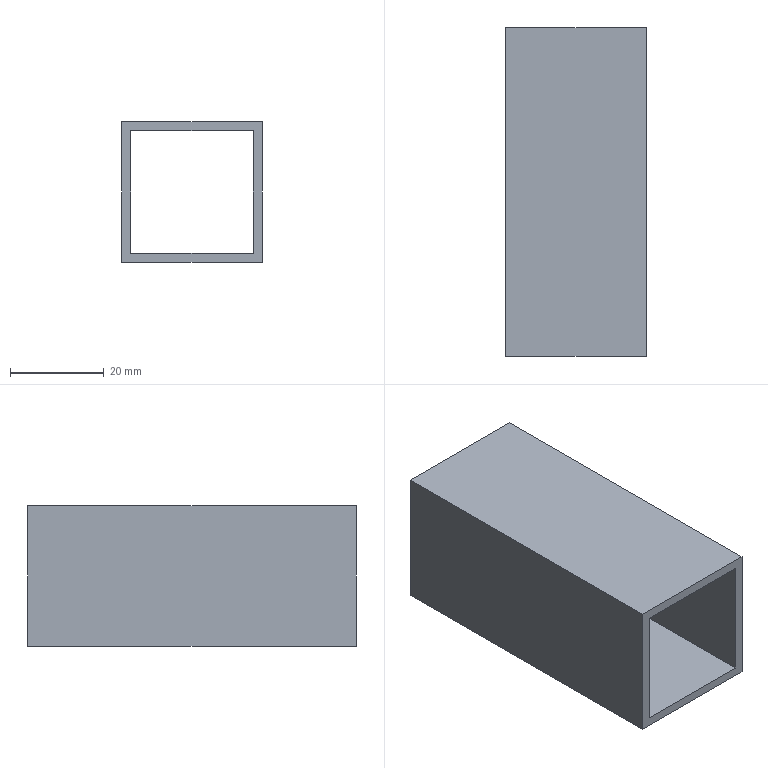Part | NX | features solid 2 | 1 solid | 10 faces | box 30 x 70 x 30 mm | volume 15680 mm3 | plane 10
STEP:
#1=CARTESIAN_POINT('',(245.839,786.479,-180.));
#2=VERTEX_POINT('',#1);
#3=CARTESIAN_POINT('',(245.839,786.479,-150.));
#4=VERTEX_POINT('',#3);
#5=CARTESIAN_POINT('',(245.839,786.479,-180.));
#6=DIRECTION('',(0.,0.,1.));
#7=VECTOR('',#6,1000.);
#8=LINE('',#5,#7);
#9=EDGE_CURVE('',#2,#4,#8,.T.);
#10=ORIENTED_EDGE('',*,*,#9,.F.);
#11=CARTESIAN_POINT('',(245.839,716.479,-180.));
#12=VERTEX_POINT('',#11);
#13=CARTESIAN_POINT('',(245.839,776.479,-180.));
#14=DIRECTION('',(0.,1.,0.));
#15=VECTOR('',#14,1000.);
#16=LINE('',#13,#15);
#17=EDGE_CURVE('',#12,#2,#16,.T.);
#18=ORIENTED_EDGE('',*,*,#17,.F.);
#19=CARTESIAN_POINT('',(245.839,716.479,-150.));
#20=VERTEX_POINT('',#19);
#21=CARTESIAN_POINT('',(245.839,716.479,-180.));
#22=DIRECTION('',(0.,0.,-1.));
#23=VECTOR('',#22,1000.);
#24=LINE('',#21,#23);
#25=EDGE_CURVE('',#12,#20,#24,.F.);
#26=ORIENTED_EDGE('',*,*,#25,.T.);
#27=CARTESIAN_POINT('',(245.839,776.479,-150.));
#28=DIRECTION('',(0.,1.,0.));
#29=VECTOR('',#28,1000.);
#30=LINE('',#27,#29);
#31=EDGE_CURVE('',#20,#4,#30,.T.);
#32=ORIENTED_EDGE('',*,*,#31,.T.);
#33=EDGE_LOOP('',(#10,#18,#26,#32));
#34=FACE_BOUND('',#33,.T.);
#35=CARTESIAN_POINT('',(245.839,776.479,-180.));
#36=DIRECTION('',(1.,0.,0.));
#37=DIRECTION('',(0.,1.,0.));
#38=AXIS2_PLACEMENT_3D('',#35,#36,#37);
#39=PLANE('',#38);
#40=ADVANCED_FACE('',(#34),#39,.F.);
#41=CARTESIAN_POINT('',(275.839,786.479,-150.));
#42=VERTEX_POINT('',#41);
#43=CARTESIAN_POINT('',(275.839,786.479,-180.));
#44=VERTEX_POINT('',#43);
#45=CARTESIAN_POINT('',(275.839,786.479,-180.));
#46=DIRECTION('',(0.,0.,1.));
#47=VECTOR('',#46,1000.);
#48=LINE('',#45,#47);
#49=EDGE_CURVE('',#42,#44,#48,.F.);
#50=ORIENTED_EDGE('',*,*,#49,.F.);
#51=CARTESIAN_POINT('',(275.839,716.479,-150.));
#52=VERTEX_POINT('',#51);
#53=CARTESIAN_POINT('',(275.839,776.479,-150.));
#54=DIRECTION('',(0.,-1.,0.));
#55=VECTOR('',#54,1000.);
#56=LINE('',#53,#55);
#57=EDGE_CURVE('',#52,#42,#56,.F.);
#58=ORIENTED_EDGE('',*,*,#57,.F.);
#59=CARTESIAN_POINT('',(275.839,716.479,-180.));
#60=VERTEX_POINT('',#59);
#61=CARTESIAN_POINT('',(275.839,716.479,-180.));
#62=DIRECTION('',(0.,0.,-1.));
#63=VECTOR('',#62,1000.);
#64=LINE('',#61,#63);
#65=EDGE_CURVE('',#52,#60,#64,.T.);
#66=ORIENTED_EDGE('',*,*,#65,.T.);
#67=CARTESIAN_POINT('',(275.839,776.479,-180.));
#68=DIRECTION('',(0.,1.,0.));
#69=VECTOR('',#68,1000.);
#70=LINE('',#67,#69);
#71=EDGE_CURVE('',#60,#44,#70,.T.);
#72=ORIENTED_EDGE('',*,*,#71,.T.);
#73=EDGE_LOOP('',(#50,#58,#66,#72));
#74=FACE_BOUND('',#73,.T.);
#75=CARTESIAN_POINT('',(275.839,776.479,-180.));
#76=DIRECTION('',(1.,0.,0.));
#77=DIRECTION('',(0.,1.,0.));
#78=AXIS2_PLACEMENT_3D('',#75,#76,#77);
#79=PLANE('',#78);
#80=ADVANCED_FACE('',(#74),#79,.T.);
#81=CARTESIAN_POINT('',(275.839,786.479,-180.));
#82=DIRECTION('',(-1.,0.,0.));
#83=VECTOR('',#82,1000.);
#84=LINE('',#81,#83);
#85=EDGE_CURVE('',#44,#2,#84,.T.);
#86=ORIENTED_EDGE('',*,*,#85,.F.);
#87=ORIENTED_EDGE('',*,*,#71,.F.);
#88=CARTESIAN_POINT('',(275.839,716.479,-180.));
#89=DIRECTION('',(1.,0.,0.));
#90=VECTOR('',#89,1000.);
#91=LINE('',#88,#90);
#92=EDGE_CURVE('',#60,#12,#91,.F.);
#93=ORIENTED_EDGE('',*,*,#92,.T.);
#94=ORIENTED_EDGE('',*,*,#17,.T.);
#95=EDGE_LOOP('',(#86,#87,#93,#94));
#96=FACE_BOUND('',#95,.T.);
#97=CARTESIAN_POINT('',(275.839,776.479,-180.));
#98=DIRECTION('',(0.,0.,1.));
#99=DIRECTION('',(0.,-1.,0.));
#100=AXIS2_PLACEMENT_3D('',#97,#98,#99);
#101=PLANE('',#100);
#102=ADVANCED_FACE('',(#96),#101,.F.);
#103=ORIENTED_EDGE('',*,*,#57,.T.);
#104=CARTESIAN_POINT('',(275.839,786.479,-150.));
#105=DIRECTION('',(-1.,0.,0.));
#106=VECTOR('',#105,1000.);
#107=LINE('',#104,#106);
#108=EDGE_CURVE('',#42,#4,#107,.T.);
#109=ORIENTED_EDGE('',*,*,#108,.T.);
#110=ORIENTED_EDGE('',*,*,#31,.F.);
#111=CARTESIAN_POINT('',(275.839,716.479,-150.));
#112=DIRECTION('',(1.,0.,0.));
#113=VECTOR('',#112,1000.);
#114=LINE('',#111,#113);
#115=EDGE_CURVE('',#52,#20,#114,.F.);
#116=ORIENTED_EDGE('',*,*,#115,.F.);
#117=EDGE_LOOP('',(#103,#109,#110,#116));
#118=FACE_BOUND('',#117,.T.);
#119=CARTESIAN_POINT('',(275.839,776.479,-150.));
#120=DIRECTION('',(0.,0.,1.));
#121=DIRECTION('',(0.,-1.,0.));
#122=AXIS2_PLACEMENT_3D('',#119,#120,#121);
#123=PLANE('',#122);
#124=ADVANCED_FACE('',(#118),#123,.T.);
#125=ORIENTED_EDGE('',*,*,#115,.T.);
#126=ORIENTED_EDGE('',*,*,#25,.F.);
#127=ORIENTED_EDGE('',*,*,#92,.F.);
#128=ORIENTED_EDGE('',*,*,#65,.F.);
#129=EDGE_LOOP('',(#125,#126,#127,#128));
#130=FACE_BOUND('',#129,.T.);
#131=CARTESIAN_POINT('',(273.839,716.479,-152.));
#132=VERTEX_POINT('',#131);
#133=CARTESIAN_POINT('',(273.839,716.479,-178.));
#134=VERTEX_POINT('',#133);
#135=CARTESIAN_POINT('',(273.839,716.479,-180.));
#136=DIRECTION('',(0.,0.,-1.));
#137=VECTOR('',#136,1000.);
#138=LINE('',#135,#137);
#139=EDGE_CURVE('',#132,#134,#138,.T.);
#140=ORIENTED_EDGE('',*,*,#139,.T.);
#141=CARTESIAN_POINT('',(247.839,716.479,-178.));
#142=VERTEX_POINT('',#141);
#143=CARTESIAN_POINT('',(275.839,716.479,-178.));
#144=DIRECTION('',(1.,0.,0.));
#145=VECTOR('',#144,1000.);
#146=LINE('',#143,#145);
#147=EDGE_CURVE('',#134,#142,#146,.F.);
#148=ORIENTED_EDGE('',*,*,#147,.T.);
#149=CARTESIAN_POINT('',(247.839,716.479,-152.));
#150=VERTEX_POINT('',#149);
#151=CARTESIAN_POINT('',(247.839,716.479,-180.));
#152=DIRECTION('',(0.,0.,-1.));
#153=VECTOR('',#152,1000.);
#154=LINE('',#151,#153);
#155=EDGE_CURVE('',#142,#150,#154,.F.);
#156=ORIENTED_EDGE('',*,*,#155,.T.);
#157=CARTESIAN_POINT('',(275.839,716.479,-152.));
#158=DIRECTION('',(1.,0.,0.));
#159=VECTOR('',#158,1000.);
#160=LINE('',#157,#159);
#161=EDGE_CURVE('',#132,#150,#160,.F.);
#162=ORIENTED_EDGE('',*,*,#161,.F.);
#163=EDGE_LOOP('',(#140,#148,#156,#162));
#164=FACE_BOUND('',#163,.T.);
#165=CARTESIAN_POINT('',(275.839,716.479,-25.));
#166=DIRECTION('',(0.,-1.,0.));
#167=DIRECTION('',(1.,0.,0.));
#168=AXIS2_PLACEMENT_3D('',#165,#166,#167);
#169=PLANE('',#168);
#170=ADVANCED_FACE('',(#130,#164),#169,.T.);
#171=CARTESIAN_POINT('',(247.839,786.479,-178.));
#172=VERTEX_POINT('',#171);
#173=CARTESIAN_POINT('',(247.839,776.479,-178.));
#174=DIRECTION('',(0.,1.,0.));
#175=VECTOR('',#174,1000.);
#176=LINE('',#173,#175);
#177=EDGE_CURVE('',#142,#172,#176,.T.);
#178=ORIENTED_EDGE('',*,*,#177,.T.);
#179=CARTESIAN_POINT('',(247.839,786.479,-152.));
#180=VERTEX_POINT('',#179);
#181=CARTESIAN_POINT('',(247.839,786.479,-180.));
#182=DIRECTION('',(0.,0.,1.));
#183=VECTOR('',#182,1000.);
#184=LINE('',#181,#183);
#185=EDGE_CURVE('',#172,#180,#184,.T.);
#186=ORIENTED_EDGE('',*,*,#185,.T.);
#187=CARTESIAN_POINT('',(247.839,776.479,-152.));
#188=DIRECTION('',(0.,1.,0.));
#189=VECTOR('',#188,1000.);
#190=LINE('',#187,#189);
#191=EDGE_CURVE('',#150,#180,#190,.T.);
#192=ORIENTED_EDGE('',*,*,#191,.F.);
#193=ORIENTED_EDGE('',*,*,#155,.F.);
#194=EDGE_LOOP('',(#178,#186,#192,#193));
#195=FACE_BOUND('',#194,.T.);
#196=CARTESIAN_POINT('',(247.839,776.479,-180.));
#197=DIRECTION('',(1.,0.,0.));
#198=DIRECTION('',(0.,1.,0.));
#199=AXIS2_PLACEMENT_3D('',#196,#197,#198);
#200=PLANE('',#199);
#201=ADVANCED_FACE('',(#195),#200,.T.);
#202=CARTESIAN_POINT('',(273.839,786.479,-152.));
#203=VERTEX_POINT('',#202);
#204=CARTESIAN_POINT('',(273.839,776.479,-152.));
#205=DIRECTION('',(0.,-1.,0.));
#206=VECTOR('',#205,1000.);
#207=LINE('',#204,#206);
#208=EDGE_CURVE('',#132,#203,#207,.F.);
#209=ORIENTED_EDGE('',*,*,#208,.T.);
#210=CARTESIAN_POINT('',(273.839,786.479,-178.));
#211=VERTEX_POINT('',#210);
#212=CARTESIAN_POINT('',(273.839,786.479,-180.));
#213=DIRECTION('',(0.,0.,1.));
#214=VECTOR('',#213,1000.);
#215=LINE('',#212,#214);
#216=EDGE_CURVE('',#203,#211,#215,.F.);
#217=ORIENTED_EDGE('',*,*,#216,.T.);
#218=CARTESIAN_POINT('',(273.839,776.479,-178.));
#219=DIRECTION('',(0.,-1.,0.));
#220=VECTOR('',#219,1000.);
#221=LINE('',#218,#220);
#222=EDGE_CURVE('',#134,#211,#221,.F.);
#223=ORIENTED_EDGE('',*,*,#222,.F.);
#224=ORIENTED_EDGE('',*,*,#139,.F.);
#225=EDGE_LOOP('',(#209,#217,#223,#224));
#226=FACE_BOUND('',#225,.T.);
#227=CARTESIAN_POINT('',(273.839,776.479,-180.));
#228=DIRECTION('',(1.,0.,0.));
#229=DIRECTION('',(0.,1.,0.));
#230=AXIS2_PLACEMENT_3D('',#227,#228,#229);
#231=PLANE('',#230);
#232=ADVANCED_FACE('',(#226),#231,.F.);
#233=ORIENTED_EDGE('',*,*,#222,.T.);
#234=CARTESIAN_POINT('',(275.839,786.479,-178.));
#235=DIRECTION('',(-1.,0.,0.));
#236=VECTOR('',#235,1000.);
#237=LINE('',#234,#236);
#238=EDGE_CURVE('',#211,#172,#237,.T.);
#239=ORIENTED_EDGE('',*,*,#238,.T.);
#240=ORIENTED_EDGE('',*,*,#177,.F.);
#241=ORIENTED_EDGE('',*,*,#147,.F.);
#242=EDGE_LOOP('',(#233,#239,#240,#241));
#243=FACE_BOUND('',#242,.T.);
#244=CARTESIAN_POINT('',(275.839,776.479,-178.));
#245=DIRECTION('',(0.,0.,1.));
#246=DIRECTION('',(0.,-1.,0.));
#247=AXIS2_PLACEMENT_3D('',#244,#245,#246);
#248=PLANE('',#247);
#249=ADVANCED_FACE('',(#243),#248,.T.);
#250=CARTESIAN_POINT('',(275.839,786.479,-152.));
#251=DIRECTION('',(-1.,0.,0.));
#252=VECTOR('',#251,1000.);
#253=LINE('',#250,#252);
#254=EDGE_CURVE('',#203,#180,#253,.T.);
#255=ORIENTED_EDGE('',*,*,#254,.F.);
#256=ORIENTED_EDGE('',*,*,#208,.F.);
#257=ORIENTED_EDGE('',*,*,#161,.T.);
#258=ORIENTED_EDGE('',*,*,#191,.T.);
#259=EDGE_LOOP('',(#255,#256,#257,#258));
#260=FACE_BOUND('',#259,.T.);
#261=CARTESIAN_POINT('',(275.839,776.479,-152.));
#262=DIRECTION('',(0.,0.,1.));
#263=DIRECTION('',(0.,-1.,0.));
#264=AXIS2_PLACEMENT_3D('',#261,#262,#263);
#265=PLANE('',#264);
#266=ADVANCED_FACE('',(#260),#265,.F.);
#267=ORIENTED_EDGE('',*,*,#185,.F.);
#268=ORIENTED_EDGE('',*,*,#238,.F.);
#269=ORIENTED_EDGE('',*,*,#216,.F.);
#270=ORIENTED_EDGE('',*,*,#254,.T.);
#271=EDGE_LOOP('',(#267,#268,#269,#270));
#272=FACE_BOUND('',#271,.T.);
#273=ORIENTED_EDGE('',*,*,#85,.T.);
#274=ORIENTED_EDGE('',*,*,#9,.T.);
#275=ORIENTED_EDGE('',*,*,#108,.F.);
#276=ORIENTED_EDGE('',*,*,#49,.T.);
#277=EDGE_LOOP('',(#273,#274,#275,#276));
#278=FACE_BOUND('',#277,.T.);
#279=CARTESIAN_POINT('',(245.839,786.479,-150.));
#280=DIRECTION('',(0.,1.,0.));
#281=DIRECTION('',(-1.,0.,0.));
#282=AXIS2_PLACEMENT_3D('',#279,#280,#281);
#283=PLANE('',#282);
#284=ADVANCED_FACE('',(#272,#278),#283,.T.);
#285=CLOSED_SHELL('',(#40,#80,#102,#124,#170,#201,#232,#249,#266,#284));
#286=MANIFOLD_SOLID_BREP('',#285);
#287=(LENGTH_UNIT()NAMED_UNIT(*)SI_UNIT(.MILLI.,.METRE.));
#288=UNCERTAINTY_MEASURE_WITH_UNIT(LENGTH_MEASURE(0.00001),#287,'','');
#289=(NAMED_UNIT(*)PLANE_ANGLE_UNIT()SI_UNIT($,.RADIAN.));
#290=(NAMED_UNIT(*)SI_UNIT($,.STERADIAN.)SOLID_ANGLE_UNIT());
#291=(GEOMETRIC_REPRESENTATION_CONTEXT(3)GLOBAL_UNCERTAINTY_ASSIGNED_CONTEXT((#288))GLOBAL_UNIT_ASSIGNED_CONTEXT((#287,#289,#290))REPRESENTATION_CONTEXT('',''));
#292=ADVANCED_BREP_SHAPE_REPRESENTATION('',(#286),#291);